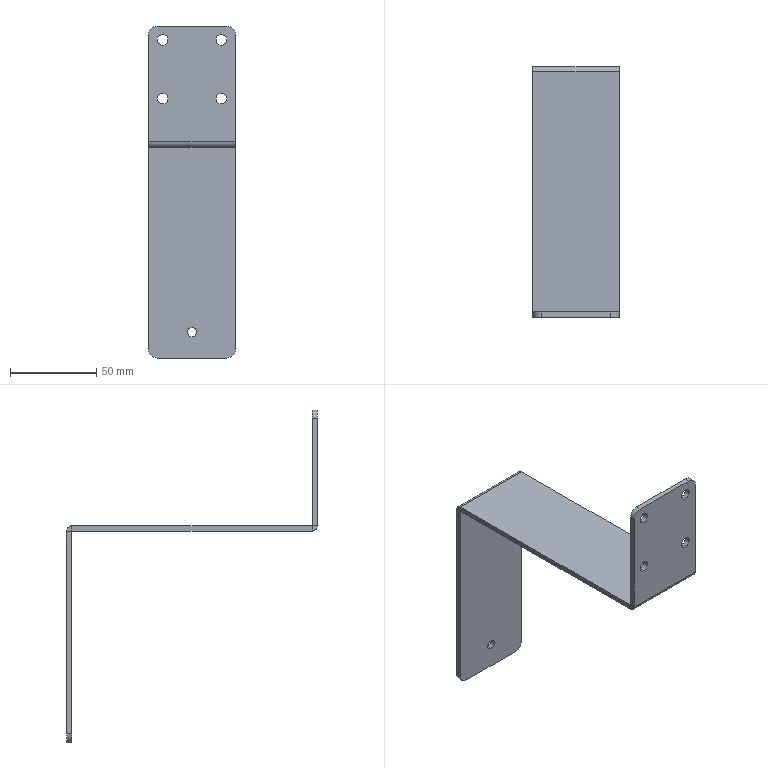Part | SolidWorks | features EdgeFlange 2, HoleWzd 2, Fillet 1, FlatPattern 1, SMBaseFlange 1, SheetMetal 1 | 1 solid | 36 faces | box 50 x 145 x 192 mm | volume 49401 mm3 | cylinder 18 | plane 18 | commonest cylinder face diameters 6.2 x10 10 x4 0.2 x2 5.3 x2
STEP:
#1=CARTESIAN_POINT('',(0.,139.,-139.35));
#2=VERTEX_POINT('',#1);
#3=CARTESIAN_POINT('',(0.,139.,-144.65));
#4=VERTEX_POINT('',#3);
#5=CARTESIAN_POINT('',(0.,139.,-142.));
#6=DIRECTION('',(0.,-1.,0.));
#7=DIRECTION('',(0.,0.,-1.));
#8=AXIS2_PLACEMENT_3D('',#5,#6,#7);
#9=CIRCLE('',#8,2.65);
#10=EDGE_CURVE('',#2,#4,#9,.T.);
#11=ORIENTED_EDGE('',*,*,#10,.T.);
#12=CARTESIAN_POINT('',(0.,142.,-144.65));
#13=VERTEX_POINT('',#12);
#14=CARTESIAN_POINT('',(0.,142.,-144.65));
#15=DIRECTION('',(0.,1.,0.));
#16=VECTOR('',#15,1000.);
#17=LINE('',#14,#16);
#18=EDGE_CURVE('',#4,#13,#17,.T.);
#19=ORIENTED_EDGE('',*,*,#18,.T.);
#20=CARTESIAN_POINT('',(0.,142.,-139.35));
#21=VERTEX_POINT('',#20);
#22=CARTESIAN_POINT('',(0.,142.,-142.));
#23=DIRECTION('',(0.,1.,0.));
#24=DIRECTION('',(0.,0.,1.));
#25=AXIS2_PLACEMENT_3D('',#22,#23,#24);
#26=CIRCLE('',#25,2.65);
#27=EDGE_CURVE('',#13,#21,#26,.T.);
#28=ORIENTED_EDGE('',*,*,#27,.T.);
#29=CARTESIAN_POINT('',(0.,142.,-139.35));
#30=DIRECTION('',(0.,1.,0.));
#31=VECTOR('',#30,1000.);
#32=LINE('',#29,#31);
#33=EDGE_CURVE('',#2,#21,#32,.T.);
#34=ORIENTED_EDGE('',*,*,#33,.F.);
#35=EDGE_LOOP('',(#11,#19,#28,#34));
#36=FACE_OUTER_BOUND('',#35,.T.);
#37=CARTESIAN_POINT('',(0.,142.,-142.));
#38=DIRECTION('',(0.,1.,0.));
#39=DIRECTION('',(0.,0.,1.));
#40=AXIS2_PLACEMENT_3D('',#37,#38,#39);
#41=CYLINDRICAL_SURFACE('',#40,2.65);
#42=ADVANCED_FACE('',(#36),#41,.F.);
#43=CARTESIAN_POINT('',(-17.,-3.,-3.9));
#44=VERTEX_POINT('',#43);
#45=CARTESIAN_POINT('',(-17.,-3.,-10.1));
#46=VERTEX_POINT('',#45);
#47=CARTESIAN_POINT('',(-17.,-3.,-7.));
#48=DIRECTION('',(0.,-1.,0.));
#49=DIRECTION('',(0.,0.,-1.));
#50=AXIS2_PLACEMENT_3D('',#47,#48,#49);
#51=CIRCLE('',#50,3.1);
#52=EDGE_CURVE('',#44,#46,#51,.T.);
#53=ORIENTED_EDGE('',*,*,#52,.T.);
#54=CARTESIAN_POINT('',(-17.,0.,-10.1));
#55=VERTEX_POINT('',#54);
#56=CARTESIAN_POINT('',(-17.,0.,-10.1));
#57=DIRECTION('',(0.,1.,0.));
#58=VECTOR('',#57,1000.);
#59=LINE('',#56,#58);
#60=EDGE_CURVE('',#46,#55,#59,.T.);
#61=ORIENTED_EDGE('',*,*,#60,.T.);
#62=CARTESIAN_POINT('',(-17.,0.,-3.9));
#63=VERTEX_POINT('',#62);
#64=CARTESIAN_POINT('',(-17.,0.,-7.));
#65=DIRECTION('',(0.,1.,0.));
#66=DIRECTION('',(0.,0.,1.));
#67=AXIS2_PLACEMENT_3D('',#64,#65,#66);
#68=CIRCLE('',#67,3.1);
#69=EDGE_CURVE('',#55,#63,#68,.T.);
#70=ORIENTED_EDGE('',*,*,#69,.T.);
#71=CARTESIAN_POINT('',(-17.,0.,-3.9));
#72=DIRECTION('',(0.,1.,0.));
#73=VECTOR('',#72,1000.);
#74=LINE('',#71,#73);
#75=EDGE_CURVE('',#44,#63,#74,.T.);
#76=ORIENTED_EDGE('',*,*,#75,.F.);
#77=EDGE_LOOP('',(#53,#61,#70,#76));
#78=FACE_OUTER_BOUND('',#77,.T.);
#79=CARTESIAN_POINT('',(-17.,0.,-7.));
#80=DIRECTION('',(0.,1.,0.));
#81=DIRECTION('',(0.,0.,1.));
#82=AXIS2_PLACEMENT_3D('',#79,#80,#81);
#83=CYLINDRICAL_SURFACE('',#82,3.1);
#84=ADVANCED_FACE('',(#78),#83,.F.);
#85=CARTESIAN_POINT('',(-17.,-3.,30.1));
#86=VERTEX_POINT('',#85);
#87=CARTESIAN_POINT('',(-17.,-3.,23.9));
#88=VERTEX_POINT('',#87);
#89=CARTESIAN_POINT('',(-17.,-3.,27.));
#90=DIRECTION('',(0.,-1.,0.));
#91=DIRECTION('',(0.,0.,-1.));
#92=AXIS2_PLACEMENT_3D('',#89,#90,#91);
#93=CIRCLE('',#92,3.1);
#94=EDGE_CURVE('',#86,#88,#93,.T.);
#95=ORIENTED_EDGE('',*,*,#94,.T.);
#96=CARTESIAN_POINT('',(-17.,0.,23.9));
#97=VERTEX_POINT('',#96);
#98=CARTESIAN_POINT('',(-17.,0.,23.9));
#99=DIRECTION('',(0.,1.,0.));
#100=VECTOR('',#99,1000.);
#101=LINE('',#98,#100);
#102=EDGE_CURVE('',#88,#97,#101,.T.);
#103=ORIENTED_EDGE('',*,*,#102,.T.);
#104=CARTESIAN_POINT('',(-17.,0.,30.1));
#105=VERTEX_POINT('',#104);
#106=CARTESIAN_POINT('',(-17.,0.,27.));
#107=DIRECTION('',(0.,1.,0.));
#108=DIRECTION('',(0.,0.,1.));
#109=AXIS2_PLACEMENT_3D('',#106,#107,#108);
#110=CIRCLE('',#109,3.1);
#111=EDGE_CURVE('',#97,#105,#110,.T.);
#112=ORIENTED_EDGE('',*,*,#111,.T.);
#113=CARTESIAN_POINT('',(-17.,0.,30.1));
#114=DIRECTION('',(0.,1.,0.));
#115=VECTOR('',#114,1000.);
#116=LINE('',#113,#115);
#117=EDGE_CURVE('',#86,#105,#116,.T.);
#118=ORIENTED_EDGE('',*,*,#117,.F.);
#119=EDGE_LOOP('',(#95,#103,#112,#118));
#120=FACE_OUTER_BOUND('',#119,.T.);
#121=CARTESIAN_POINT('',(-17.,0.,27.));
#122=DIRECTION('',(0.,1.,0.));
#123=DIRECTION('',(0.,0.,1.));
#124=AXIS2_PLACEMENT_3D('',#121,#122,#123);
#125=CYLINDRICAL_SURFACE('',#124,3.1);
#126=ADVANCED_FACE('',(#120),#125,.F.);
#127=CARTESIAN_POINT('',(17.,-3.,30.1));
#128=VERTEX_POINT('',#127);
#129=CARTESIAN_POINT('',(17.,-3.,23.9));
#130=VERTEX_POINT('',#129);
#131=CARTESIAN_POINT('',(17.,-3.,27.));
#132=DIRECTION('',(0.,-1.,0.));
#133=DIRECTION('',(0.,0.,-1.));
#134=AXIS2_PLACEMENT_3D('',#131,#132,#133);
#135=CIRCLE('',#134,3.1);
#136=EDGE_CURVE('',#128,#130,#135,.T.);
#137=ORIENTED_EDGE('',*,*,#136,.T.);
#138=CARTESIAN_POINT('',(17.,0.,23.9));
#139=VERTEX_POINT('',#138);
#140=CARTESIAN_POINT('',(17.,0.,23.9));
#141=DIRECTION('',(0.,1.,0.));
#142=VECTOR('',#141,1000.);
#143=LINE('',#140,#142);
#144=EDGE_CURVE('',#130,#139,#143,.T.);
#145=ORIENTED_EDGE('',*,*,#144,.T.);
#146=CARTESIAN_POINT('',(17.,0.,30.1));
#147=VERTEX_POINT('',#146);
#148=CARTESIAN_POINT('',(17.,0.,27.));
#149=DIRECTION('',(0.,1.,0.));
#150=DIRECTION('',(0.,0.,1.));
#151=AXIS2_PLACEMENT_3D('',#148,#149,#150);
#152=CIRCLE('',#151,3.1);
#153=EDGE_CURVE('',#139,#147,#152,.T.);
#154=ORIENTED_EDGE('',*,*,#153,.T.);
#155=CARTESIAN_POINT('',(17.,0.,30.1));
#156=DIRECTION('',(0.,1.,0.));
#157=VECTOR('',#156,1000.);
#158=LINE('',#155,#157);
#159=EDGE_CURVE('',#128,#147,#158,.T.);
#160=ORIENTED_EDGE('',*,*,#159,.F.);
#161=EDGE_LOOP('',(#137,#145,#154,#160));
#162=FACE_OUTER_BOUND('',#161,.T.);
#163=CARTESIAN_POINT('',(17.,0.,27.));
#164=DIRECTION('',(0.,1.,0.));
#165=DIRECTION('',(0.,0.,1.));
#166=AXIS2_PLACEMENT_3D('',#163,#164,#165);
#167=CYLINDRICAL_SURFACE('',#166,3.1);
#168=ADVANCED_FACE('',(#162),#167,.F.);
#169=CARTESIAN_POINT('',(17.,-3.,-3.9));
#170=VERTEX_POINT('',#169);
#171=CARTESIAN_POINT('',(17.,-3.,-10.1));
#172=VERTEX_POINT('',#171);
#173=CARTESIAN_POINT('',(17.,-3.,-7.));
#174=DIRECTION('',(0.,-1.,0.));
#175=DIRECTION('',(0.,0.,-1.));
#176=AXIS2_PLACEMENT_3D('',#173,#174,#175);
#177=CIRCLE('',#176,3.1);
#178=EDGE_CURVE('',#170,#172,#177,.T.);
#179=ORIENTED_EDGE('',*,*,#178,.T.);
#180=CARTESIAN_POINT('',(17.,0.,-10.1));
#181=VERTEX_POINT('',#180);
#182=CARTESIAN_POINT('',(17.,0.,-10.1));
#183=DIRECTION('',(0.,1.,0.));
#184=VECTOR('',#183,1000.);
#185=LINE('',#182,#184);
#186=EDGE_CURVE('',#172,#181,#185,.T.);
#187=ORIENTED_EDGE('',*,*,#186,.T.);
#188=CARTESIAN_POINT('',(17.,0.,-3.9));
#189=VERTEX_POINT('',#188);
#190=CARTESIAN_POINT('',(17.,0.,-7.));
#191=DIRECTION('',(0.,1.,0.));
#192=DIRECTION('',(0.,0.,1.));
#193=AXIS2_PLACEMENT_3D('',#190,#191,#192);
#194=CIRCLE('',#193,3.1);
#195=EDGE_CURVE('',#181,#189,#194,.T.);
#196=ORIENTED_EDGE('',*,*,#195,.T.);
#197=CARTESIAN_POINT('',(17.,0.,-3.9));
#198=DIRECTION('',(0.,1.,0.));
#199=VECTOR('',#198,1000.);
#200=LINE('',#197,#199);
#201=EDGE_CURVE('',#170,#189,#200,.T.);
#202=ORIENTED_EDGE('',*,*,#201,.F.);
#203=EDGE_LOOP('',(#179,#187,#196,#202));
#204=FACE_OUTER_BOUND('',#203,.T.);
#205=CARTESIAN_POINT('',(17.,0.,-7.));
#206=DIRECTION('',(0.,1.,0.));
#207=DIRECTION('',(0.,0.,1.));
#208=AXIS2_PLACEMENT_3D('',#205,#206,#207);
#209=CYLINDRICAL_SURFACE('',#208,3.1);
#210=ADVANCED_FACE('',(#204),#209,.F.);
#211=CARTESIAN_POINT('',(25.,138.9,-35.));
#212=VERTEX_POINT('',#211);
#213=CARTESIAN_POINT('',(25.,138.9,-32.));
#214=VERTEX_POINT('',#213);
#215=CARTESIAN_POINT('',(25.,138.9,-35.));
#216=DIRECTION('',(0.,0.,1.));
#217=VECTOR('',#216,1000.);
#218=LINE('',#215,#217);
#219=EDGE_CURVE('',#212,#214,#218,.T.);
#220=ORIENTED_EDGE('',*,*,#219,.T.);
#221=CARTESIAN_POINT('',(25.,0.1,-32.));
#222=VERTEX_POINT('',#221);
#223=CARTESIAN_POINT('',(25.,0.,-32.));
#224=DIRECTION('',(0.,-1.,0.));
#225=VECTOR('',#224,1000.);
#226=LINE('',#223,#225);
#227=EDGE_CURVE('',#214,#222,#226,.T.);
#228=ORIENTED_EDGE('',*,*,#227,.T.);
#229=CARTESIAN_POINT('',(25.,0.1,-35.));
#230=VERTEX_POINT('',#229);
#231=CARTESIAN_POINT('',(25.,0.1,-35.));
#232=DIRECTION('',(0.,0.,-1.));
#233=VECTOR('',#232,1000.);
#234=LINE('',#231,#233);
#235=EDGE_CURVE('',#222,#230,#234,.T.);
#236=ORIENTED_EDGE('',*,*,#235,.T.);
#237=CARTESIAN_POINT('',(25.,0.,-35.));
#238=DIRECTION('',(0.,-1.,0.));
#239=VECTOR('',#238,1000.);
#240=LINE('',#237,#239);
#241=EDGE_CURVE('',#212,#230,#240,.T.);
#242=ORIENTED_EDGE('',*,*,#241,.F.);
#243=EDGE_LOOP('',(#220,#228,#236,#242));
#244=FACE_OUTER_BOUND('',#243,.T.);
#245=CARTESIAN_POINT('',(25.,0.,-35.));
#246=DIRECTION('',(-1.,0.,0.));
#247=DIRECTION('',(0.,-1.,0.));
#248=AXIS2_PLACEMENT_3D('',#245,#246,#247);
#249=PLANE('',#248);
#250=ADVANCED_FACE('',(#244),#249,.F.);
#251=CARTESIAN_POINT('',(-25.,138.9,-35.));
#252=VERTEX_POINT('',#251);
#253=CARTESIAN_POINT('',(-25.,138.9,-32.));
#254=VERTEX_POINT('',#253);
#255=CARTESIAN_POINT('',(-25.,138.9,-35.));
#256=DIRECTION('',(0.,0.,1.));
#257=VECTOR('',#256,1000.);
#258=LINE('',#255,#257);
#259=EDGE_CURVE('',#252,#254,#258,.T.);
#260=ORIENTED_EDGE('',*,*,#259,.F.);
#261=CARTESIAN_POINT('',(-25.,0.1,-35.));
#262=VERTEX_POINT('',#261);
#263=CARTESIAN_POINT('',(-25.,0.,-35.));
#264=DIRECTION('',(0.,1.,0.));
#265=VECTOR('',#264,1000.);
#266=LINE('',#263,#265);
#267=EDGE_CURVE('',#262,#252,#266,.T.);
#268=ORIENTED_EDGE('',*,*,#267,.F.);
#269=CARTESIAN_POINT('',(-25.,0.1,-32.));
#270=VERTEX_POINT('',#269);
#271=CARTESIAN_POINT('',(-25.,0.1,-32.));
#272=DIRECTION('',(0.,0.,-1.));
#273=VECTOR('',#272,1000.);
#274=LINE('',#271,#273);
#275=EDGE_CURVE('',#270,#262,#274,.T.);
#276=ORIENTED_EDGE('',*,*,#275,.F.);
#277=CARTESIAN_POINT('',(-25.,142.,-32.));
#278=DIRECTION('',(0.,1.,0.));
#279=VECTOR('',#278,1000.);
#280=LINE('',#277,#279);
#281=EDGE_CURVE('',#270,#254,#280,.T.);
#282=ORIENTED_EDGE('',*,*,#281,.T.);
#283=EDGE_LOOP('',(#260,#268,#276,#282));
#284=FACE_OUTER_BOUND('',#283,.T.);
#285=CARTESIAN_POINT('',(-25.,142.,-35.));
#286=DIRECTION('',(1.,0.,0.));
#287=DIRECTION('',(0.,1.,0.));
#288=AXIS2_PLACEMENT_3D('',#285,#286,#287);
#289=PLANE('',#288);
#290=ADVANCED_FACE('',(#284),#289,.F.);
#291=CARTESIAN_POINT('',(25.,138.9,-35.));
#292=DIRECTION('',(-1.,0.,0.));
#293=VECTOR('',#292,1000.);
#294=LINE('',#291,#293);
#295=EDGE_CURVE('',#212,#252,#294,.T.);
#296=ORIENTED_EDGE('',*,*,#295,.F.);
#297=ORIENTED_EDGE('',*,*,#241,.T.);
#298=CARTESIAN_POINT('',(25.,0.1,-35.));
#299=DIRECTION('',(1.,0.,0.));
#300=VECTOR('',#299,1000.);
#301=LINE('',#298,#300);
#302=EDGE_CURVE('',#262,#230,#301,.T.);
#303=ORIENTED_EDGE('',*,*,#302,.F.);
#304=ORIENTED_EDGE('',*,*,#267,.T.);
#305=EDGE_LOOP('',(#296,#297,#303,#304));
#306=FACE_OUTER_BOUND('',#305,.T.);
#307=CARTESIAN_POINT('',(0.,0.,-35.));
#308=DIRECTION('',(0.,0.,1.));
#309=DIRECTION('',(0.,-1.,0.));
#310=AXIS2_PLACEMENT_3D('',#307,#308,#309);
#311=PLANE('',#310);
#312=ADVANCED_FACE('',(#306),#311,.F.);
#313=ORIENTED_EDGE('',*,*,#227,.F.);
#314=CARTESIAN_POINT('',(25.,138.9,-32.));
#315=DIRECTION('',(-1.,0.,0.));
#316=VECTOR('',#315,1000.);
#317=LINE('',#314,#316);
#318=EDGE_CURVE('',#214,#254,#317,.T.);
#319=ORIENTED_EDGE('',*,*,#318,.T.);
#320=ORIENTED_EDGE('',*,*,#281,.F.);
#321=CARTESIAN_POINT('',(25.,0.1,-32.));
#322=DIRECTION('',(-1.,0.,0.));
#323=VECTOR('',#322,1000.);
#324=LINE('',#321,#323);
#325=EDGE_CURVE('',#222,#270,#324,.T.);
#326=ORIENTED_EDGE('',*,*,#325,.F.);
#327=EDGE_LOOP('',(#313,#319,#320,#326));
#328=FACE_OUTER_BOUND('',#327,.T.);
#329=CARTESIAN_POINT('',(0.,0.,-32.));
#330=DIRECTION('',(0.,0.,1.));
#331=DIRECTION('',(0.,-1.,0.));
#332=AXIS2_PLACEMENT_3D('',#329,#330,#331);
#333=PLANE('',#332);
#334=ADVANCED_FACE('',(#328),#333,.T.);
#335=CARTESIAN_POINT('',(-17.,0.,27.));
#336=DIRECTION('',(0.,1.,0.));
#337=DIRECTION('',(0.,0.,1.));
#338=AXIS2_PLACEMENT_3D('',#335,#336,#337);
#339=CIRCLE('',#338,3.1);
#340=EDGE_CURVE('',#105,#97,#339,.T.);
#341=ORIENTED_EDGE('',*,*,#340,.F.);
#342=ORIENTED_EDGE('',*,*,#111,.F.);
#343=EDGE_LOOP('',(#341,#342));
#344=FACE_BOUND('',#343,.T.);
#345=CARTESIAN_POINT('',(17.,0.,-7.));
#346=DIRECTION('',(0.,1.,0.));
#347=DIRECTION('',(0.,0.,1.));
#348=AXIS2_PLACEMENT_3D('',#345,#346,#347);
#349=CIRCLE('',#348,3.1);
#350=EDGE_CURVE('',#189,#181,#349,.T.);
#351=ORIENTED_EDGE('',*,*,#350,.F.);
#352=ORIENTED_EDGE('',*,*,#195,.F.);
#353=EDGE_LOOP('',(#351,#352));
#354=FACE_BOUND('',#353,.T.);
#355=CARTESIAN_POINT('',(17.,0.,27.));
#356=DIRECTION('',(0.,1.,0.));
#357=DIRECTION('',(0.,0.,1.));
#358=AXIS2_PLACEMENT_3D('',#355,#356,#357);
#359=CIRCLE('',#358,3.1);
#360=EDGE_CURVE('',#147,#139,#359,.T.);
#361=ORIENTED_EDGE('',*,*,#360,.F.);
#362=ORIENTED_EDGE('',*,*,#153,.F.);
#363=EDGE_LOOP('',(#361,#362));
#364=FACE_BOUND('',#363,.T.);
#365=CARTESIAN_POINT('',(-17.,0.,-7.));
#366=DIRECTION('',(0.,1.,0.));
#367=DIRECTION('',(0.,0.,1.));
#368=AXIS2_PLACEMENT_3D('',#365,#366,#367);
#369=CIRCLE('',#368,3.1);
#370=EDGE_CURVE('',#63,#55,#369,.T.);
#371=ORIENTED_EDGE('',*,*,#370,.F.);
#372=ORIENTED_EDGE('',*,*,#69,.F.);
#373=EDGE_LOOP('',(#371,#372));
#374=FACE_BOUND('',#373,.T.);
#375=CARTESIAN_POINT('',(-20.,0.,35.));
#376=VERTEX_POINT('',#375);
#377=CARTESIAN_POINT('',(20.,0.,35.));
#378=VERTEX_POINT('',#377);
#379=CARTESIAN_POINT('',(-25.,0.,35.));
#380=DIRECTION('',(1.,0.,0.));
#381=VECTOR('',#380,1000.);
#382=LINE('',#379,#381);
#383=EDGE_CURVE('',#376,#378,#382,.T.);
#384=ORIENTED_EDGE('',*,*,#383,.T.);
#385=CARTESIAN_POINT('',(25.,0.,30.));
#386=VERTEX_POINT('',#385);
#387=CARTESIAN_POINT('',(20.,0.,30.));
#388=DIRECTION('',(0.,1.,0.));
#389=DIRECTION('',(0.,0.,-1.));
#390=AXIS2_PLACEMENT_3D('',#387,#388,#389);
#391=CIRCLE('',#390,5.);
#392=EDGE_CURVE('',#378,#386,#391,.T.);
#393=ORIENTED_EDGE('',*,*,#392,.T.);
#394=CARTESIAN_POINT('',(25.,0.,-31.9));
#395=VERTEX_POINT('',#394);
#396=CARTESIAN_POINT('',(25.,0.,35.));
#397=DIRECTION('',(0.,0.,-1.));
#398=VECTOR('',#397,1000.);
#399=LINE('',#396,#398);
#400=EDGE_CURVE('',#386,#395,#399,.T.);
#401=ORIENTED_EDGE('',*,*,#400,.T.);
#402=CARTESIAN_POINT('',(-25.,0.,-31.9));
#403=VERTEX_POINT('',#402);
#404=CARTESIAN_POINT('',(-25.,0.,-31.9));
#405=DIRECTION('',(1.,0.,0.));
#406=VECTOR('',#405,1000.);
#407=LINE('',#404,#406);
#408=EDGE_CURVE('',#403,#395,#407,.T.);
#409=ORIENTED_EDGE('',*,*,#408,.F.);
#410=CARTESIAN_POINT('',(-25.,0.,30.));
#411=VERTEX_POINT('',#410);
#412=CARTESIAN_POINT('',(-25.,0.,35.));
#413=DIRECTION('',(0.,0.,1.));
#414=VECTOR('',#413,1000.);
#415=LINE('',#412,#414);
#416=EDGE_CURVE('',#403,#411,#415,.T.);
#417=ORIENTED_EDGE('',*,*,#416,.T.);
#418=CARTESIAN_POINT('',(-20.,0.,30.));
#419=DIRECTION('',(0.,1.,0.));
#420=DIRECTION('',(0.,0.,-1.));
#421=AXIS2_PLACEMENT_3D('',#418,#419,#420);
#422=CIRCLE('',#421,5.);
#423=EDGE_CURVE('',#411,#376,#422,.T.);
#424=ORIENTED_EDGE('',*,*,#423,.T.);
#425=EDGE_LOOP('',(#384,#393,#401,#409,#417,#424));
#426=FACE_OUTER_BOUND('',#425,.T.);
#427=CARTESIAN_POINT('',(0.,0.,0.));
#428=DIRECTION('',(0.,-1.,0.));
#429=DIRECTION('',(0.,0.,-1.));
#430=AXIS2_PLACEMENT_3D('',#427,#428,#429);
#431=PLANE('',#430);
#432=ADVANCED_FACE('',(#344,#354,#364,#374,#426),#431,.F.);
#433=CARTESIAN_POINT('',(-25.,-3.,-31.9));
#434=VERTEX_POINT('',#433);
#435=CARTESIAN_POINT('',(-25.,-3.,30.));
#436=VERTEX_POINT('',#435);
#437=CARTESIAN_POINT('',(-25.,-3.,35.));
#438=DIRECTION('',(0.,0.,1.));
#439=VECTOR('',#438,1000.);
#440=LINE('',#437,#439);
#441=EDGE_CURVE('',#434,#436,#440,.T.);
#442=ORIENTED_EDGE('',*,*,#441,.T.);
#443=CARTESIAN_POINT('',(-25.,-3.,30.));
#444=DIRECTION('',(0.,1.,0.));
#445=VECTOR('',#444,1000.);
#446=LINE('',#443,#445);
#447=EDGE_CURVE('',#436,#411,#446,.T.);
#448=ORIENTED_EDGE('',*,*,#447,.T.);
#449=ORIENTED_EDGE('',*,*,#416,.F.);
#450=CARTESIAN_POINT('',(-25.,0.,-31.9));
#451=DIRECTION('',(0.,-1.,0.));
#452=VECTOR('',#451,1000.);
#453=LINE('',#450,#452);
#454=EDGE_CURVE('',#403,#434,#453,.T.);
#455=ORIENTED_EDGE('',*,*,#454,.T.);
#456=EDGE_LOOP('',(#442,#448,#449,#455));
#457=FACE_OUTER_BOUND('',#456,.T.);
#458=CARTESIAN_POINT('',(-25.,-3.,35.));
#459=DIRECTION('',(-1.,0.,0.));
#460=DIRECTION('',(0.,0.,1.));
#461=AXIS2_PLACEMENT_3D('',#458,#459,#460);
#462=PLANE('',#461);
#463=ADVANCED_FACE('',(#457),#462,.T.);
#464=ORIENTED_EDGE('',*,*,#52,.F.);
#465=CARTESIAN_POINT('',(-17.,-3.,-7.));
#466=DIRECTION('',(0.,-1.,0.));
#467=DIRECTION('',(0.,0.,-1.));
#468=AXIS2_PLACEMENT_3D('',#465,#466,#467);
#469=CIRCLE('',#468,3.1);
#470=EDGE_CURVE('',#46,#44,#469,.T.);
#471=ORIENTED_EDGE('',*,*,#470,.F.);
#472=EDGE_LOOP('',(#464,#471));
#473=FACE_BOUND('',#472,.T.);
#474=ORIENTED_EDGE('',*,*,#94,.F.);
#475=CARTESIAN_POINT('',(-17.,-3.,27.));
#476=DIRECTION('',(0.,-1.,0.));
#477=DIRECTION('',(0.,0.,-1.));
#478=AXIS2_PLACEMENT_3D('',#475,#476,#477);
#479=CIRCLE('',#478,3.1);
#480=EDGE_CURVE('',#88,#86,#479,.T.);
#481=ORIENTED_EDGE('',*,*,#480,.F.);
#482=EDGE_LOOP('',(#474,#481));
#483=FACE_BOUND('',#482,.T.);
#484=ORIENTED_EDGE('',*,*,#136,.F.);
#485=CARTESIAN_POINT('',(17.,-3.,27.));
#486=DIRECTION('',(0.,-1.,0.));
#487=DIRECTION('',(0.,0.,-1.));
#488=AXIS2_PLACEMENT_3D('',#485,#486,#487);
#489=CIRCLE('',#488,3.1);
#490=EDGE_CURVE('',#130,#128,#489,.T.);
#491=ORIENTED_EDGE('',*,*,#490,.F.);
#492=EDGE_LOOP('',(#484,#491));
#493=FACE_BOUND('',#492,.T.);
#494=ORIENTED_EDGE('',*,*,#178,.F.);
#495=CARTESIAN_POINT('',(17.,-3.,-7.));
#496=DIRECTION('',(0.,-1.,0.));
#497=DIRECTION('',(0.,0.,-1.));
#498=AXIS2_PLACEMENT_3D('',#495,#496,#497);
#499=CIRCLE('',#498,3.1);
#500=EDGE_CURVE('',#172,#170,#499,.T.);
#501=ORIENTED_EDGE('',*,*,#500,.F.);
#502=EDGE_LOOP('',(#494,#501));
#503=FACE_BOUND('',#502,.T.);
#504=CARTESIAN_POINT('',(25.,-3.,30.));
#505=VERTEX_POINT('',#504);
#506=CARTESIAN_POINT('',(25.,-3.,-31.9));
#507=VERTEX_POINT('',#506);
#508=CARTESIAN_POINT('',(25.,-3.,35.));
#509=DIRECTION('',(0.,0.,-1.));
#510=VECTOR('',#509,1000.);
#511=LINE('',#508,#510);
#512=EDGE_CURVE('',#505,#507,#511,.T.);
#513=ORIENTED_EDGE('',*,*,#512,.F.);
#514=CARTESIAN_POINT('',(20.,-3.,35.));
#515=VERTEX_POINT('',#514);
#516=CARTESIAN_POINT('',(20.,-3.,30.));
#517=DIRECTION('',(0.,-1.,0.));
#518=DIRECTION('',(0.,0.,-1.));
#519=AXIS2_PLACEMENT_3D('',#516,#517,#518);
#520=CIRCLE('',#519,5.);
#521=EDGE_CURVE('',#505,#515,#520,.T.);
#522=ORIENTED_EDGE('',*,*,#521,.T.);
#523=CARTESIAN_POINT('',(-20.,-3.,35.));
#524=VERTEX_POINT('',#523);
#525=CARTESIAN_POINT('',(-25.,-3.,35.));
#526=DIRECTION('',(1.,0.,0.));
#527=VECTOR('',#526,1000.);
#528=LINE('',#525,#527);
#529=EDGE_CURVE('',#524,#515,#528,.T.);
#530=ORIENTED_EDGE('',*,*,#529,.F.);
#531=CARTESIAN_POINT('',(-20.,-3.,30.));
#532=DIRECTION('',(0.,-1.,0.));
#533=DIRECTION('',(0.,0.,-1.));
#534=AXIS2_PLACEMENT_3D('',#531,#532,#533);
#535=CIRCLE('',#534,5.);
#536=EDGE_CURVE('',#524,#436,#535,.T.);
#537=ORIENTED_EDGE('',*,*,#536,.T.);
#538=ORIENTED_EDGE('',*,*,#441,.F.);
#539=CARTESIAN_POINT('',(-25.,-3.,-31.9));
#540=DIRECTION('',(1.,0.,0.));
#541=VECTOR('',#540,1000.);
#542=LINE('',#539,#541);
#543=EDGE_CURVE('',#434,#507,#542,.T.);
#544=ORIENTED_EDGE('',*,*,#543,.T.);
#545=EDGE_LOOP('',(#513,#522,#530,#537,#538,#544));
#546=FACE_OUTER_BOUND('',#545,.T.);
#547=CARTESIAN_POINT('',(0.,-3.,0.));
#548=DIRECTION('',(0.,-1.,0.));
#549=DIRECTION('',(0.,0.,-1.));
#550=AXIS2_PLACEMENT_3D('',#547,#548,#549);
#551=PLANE('',#550);
#552=ADVANCED_FACE('',(#473,#483,#493,#503,#546),#551,.T.);
#553=ORIENTED_EDGE('',*,*,#400,.F.);
#554=CARTESIAN_POINT('',(25.,-3.,30.));
#555=DIRECTION('',(0.,-1.,0.));
#556=VECTOR('',#555,1000.);
#557=LINE('',#554,#556);
#558=EDGE_CURVE('',#386,#505,#557,.T.);
#559=ORIENTED_EDGE('',*,*,#558,.T.);
#560=ORIENTED_EDGE('',*,*,#512,.T.);
#561=CARTESIAN_POINT('',(25.,0.,-31.9));
#562=DIRECTION('',(0.,-1.,0.));
#563=VECTOR('',#562,1000.);
#564=LINE('',#561,#563);
#565=EDGE_CURVE('',#395,#507,#564,.T.);
#566=ORIENTED_EDGE('',*,*,#565,.F.);
#567=EDGE_LOOP('',(#553,#559,#560,#566));
#568=FACE_OUTER_BOUND('',#567,.T.);
#569=CARTESIAN_POINT('',(25.,-3.,35.));
#570=DIRECTION('',(1.,0.,0.));
#571=DIRECTION('',(0.,0.,-1.));
#572=AXIS2_PLACEMENT_3D('',#569,#570,#571);
#573=PLANE('',#572);
#574=ADVANCED_FACE('',(#568),#573,.T.);
#575=ORIENTED_EDGE('',*,*,#529,.T.);
#576=CARTESIAN_POINT('',(20.,-3.,35.));
#577=DIRECTION('',(0.,1.,0.));
#578=VECTOR('',#577,1000.);
#579=LINE('',#576,#578);
#580=EDGE_CURVE('',#515,#378,#579,.T.);
#581=ORIENTED_EDGE('',*,*,#580,.T.);
#582=ORIENTED_EDGE('',*,*,#383,.F.);
#583=CARTESIAN_POINT('',(-20.,-3.,35.));
#584=DIRECTION('',(0.,-1.,0.));
#585=VECTOR('',#584,1000.);
#586=LINE('',#583,#585);
#587=EDGE_CURVE('',#376,#524,#586,.T.);
#588=ORIENTED_EDGE('',*,*,#587,.T.);
#589=EDGE_LOOP('',(#575,#581,#582,#588));
#590=FACE_OUTER_BOUND('',#589,.T.);
#591=CARTESIAN_POINT('',(-25.,-3.,35.));
#592=DIRECTION('',(0.,0.,1.));
#593=DIRECTION('',(1.,0.,0.));
#594=AXIS2_PLACEMENT_3D('',#591,#592,#593);
#595=PLANE('',#594);
#596=ADVANCED_FACE('',(#590),#595,.T.);
#597=ORIENTED_EDGE('',*,*,#186,.F.);
#598=ORIENTED_EDGE('',*,*,#500,.T.);
#599=ORIENTED_EDGE('',*,*,#201,.T.);
#600=ORIENTED_EDGE('',*,*,#350,.T.);
#601=EDGE_LOOP('',(#597,#598,#599,#600));
#602=FACE_OUTER_BOUND('',#601,.T.);
#603=CARTESIAN_POINT('',(17.,0.,-7.));
#604=DIRECTION('',(0.,1.,0.));
#605=DIRECTION('',(0.,0.,1.));
#606=AXIS2_PLACEMENT_3D('',#603,#604,#605);
#607=CYLINDRICAL_SURFACE('',#606,3.1);
#608=ADVANCED_FACE('',(#602),#607,.F.);
#609=ORIENTED_EDGE('',*,*,#144,.F.);
#610=ORIENTED_EDGE('',*,*,#490,.T.);
#611=ORIENTED_EDGE('',*,*,#159,.T.);
#612=ORIENTED_EDGE('',*,*,#360,.T.);
#613=EDGE_LOOP('',(#609,#610,#611,#612));
#614=FACE_OUTER_BOUND('',#613,.T.);
#615=CARTESIAN_POINT('',(17.,0.,27.));
#616=DIRECTION('',(0.,1.,0.));
#617=DIRECTION('',(0.,0.,1.));
#618=AXIS2_PLACEMENT_3D('',#615,#616,#617);
#619=CYLINDRICAL_SURFACE('',#618,3.1);
#620=ADVANCED_FACE('',(#614),#619,.F.);
#621=ORIENTED_EDGE('',*,*,#102,.F.);
#622=ORIENTED_EDGE('',*,*,#480,.T.);
#623=ORIENTED_EDGE('',*,*,#117,.T.);
#624=ORIENTED_EDGE('',*,*,#340,.T.);
#625=EDGE_LOOP('',(#621,#622,#623,#624));
#626=FACE_OUTER_BOUND('',#625,.T.);
#627=CARTESIAN_POINT('',(-17.,0.,27.));
#628=DIRECTION('',(0.,1.,0.));
#629=DIRECTION('',(0.,0.,1.));
#630=AXIS2_PLACEMENT_3D('',#627,#628,#629);
#631=CYLINDRICAL_SURFACE('',#630,3.1);
#632=ADVANCED_FACE('',(#626),#631,.F.);
#633=ORIENTED_EDGE('',*,*,#60,.F.);
#634=ORIENTED_EDGE('',*,*,#470,.T.);
#635=ORIENTED_EDGE('',*,*,#75,.T.);
#636=ORIENTED_EDGE('',*,*,#370,.T.);
#637=EDGE_LOOP('',(#633,#634,#635,#636));
#638=FACE_OUTER_BOUND('',#637,.T.);
#639=CARTESIAN_POINT('',(-17.,0.,-7.));
#640=DIRECTION('',(0.,1.,0.));
#641=DIRECTION('',(0.,0.,1.));
#642=AXIS2_PLACEMENT_3D('',#639,#640,#641);
#643=CYLINDRICAL_SURFACE('',#642,3.1);
#644=ADVANCED_FACE('',(#638),#643,.F.);
#645=ORIENTED_EDGE('',*,*,#235,.F.);
#646=CARTESIAN_POINT('',(25.,0.1,-31.9));
#647=DIRECTION('',(1.,0.,0.));
#648=DIRECTION('',(0.,0.,1.));
#649=AXIS2_PLACEMENT_3D('',#646,#647,#648);
#650=CIRCLE('',#649,0.1);
#651=EDGE_CURVE('',#395,#222,#650,.T.);
#652=ORIENTED_EDGE('',*,*,#651,.F.);
#653=ORIENTED_EDGE('',*,*,#565,.T.);
#654=CARTESIAN_POINT('',(25.,0.1,-31.9));
#655=DIRECTION('',(1.,0.,0.));
#656=DIRECTION('',(0.,0.,1.));
#657=AXIS2_PLACEMENT_3D('',#654,#655,#656);
#658=CIRCLE('',#657,3.1);
#659=EDGE_CURVE('',#507,#230,#658,.T.);
#660=ORIENTED_EDGE('',*,*,#659,.T.);
#661=EDGE_LOOP('',(#645,#652,#653,#660));
#662=FACE_OUTER_BOUND('',#661,.T.);
#663=CARTESIAN_POINT('',(25.,0.1,-31.9));
#664=DIRECTION('',(1.,0.,0.));
#665=DIRECTION('',(0.,0.,-1.));
#666=AXIS2_PLACEMENT_3D('',#663,#664,#665);
#667=PLANE('',#666);
#668=ADVANCED_FACE('',(#662),#667,.T.);
#669=CARTESIAN_POINT('',(-25.,0.1,-31.9));
#670=DIRECTION('',(-1.,0.,0.));
#671=DIRECTION('',(0.,0.,1.));
#672=AXIS2_PLACEMENT_3D('',#669,#670,#671);
#673=CIRCLE('',#672,0.1);
#674=EDGE_CURVE('',#270,#403,#673,.T.);
#675=ORIENTED_EDGE('',*,*,#674,.F.);
#676=ORIENTED_EDGE('',*,*,#275,.T.);
#677=CARTESIAN_POINT('',(-25.,0.1,-31.9));
#678=DIRECTION('',(-1.,0.,0.));
#679=DIRECTION('',(0.,0.,1.));
#680=AXIS2_PLACEMENT_3D('',#677,#678,#679);
#681=CIRCLE('',#680,3.1);
#682=EDGE_CURVE('',#262,#434,#681,.T.);
#683=ORIENTED_EDGE('',*,*,#682,.T.);
#684=ORIENTED_EDGE('',*,*,#454,.F.);
#685=EDGE_LOOP('',(#675,#676,#683,#684));
#686=FACE_OUTER_BOUND('',#685,.T.);
#687=CARTESIAN_POINT('',(-25.,0.1,-31.9));
#688=DIRECTION('',(1.,0.,0.));
#689=DIRECTION('',(0.,0.,-1.));
#690=AXIS2_PLACEMENT_3D('',#687,#688,#689);
#691=PLANE('',#690);
#692=ADVANCED_FACE('',(#686),#691,.F.);
#693=ORIENTED_EDGE('',*,*,#543,.F.);
#694=ORIENTED_EDGE('',*,*,#682,.F.);
#695=ORIENTED_EDGE('',*,*,#302,.T.);
#696=ORIENTED_EDGE('',*,*,#659,.F.);
#697=EDGE_LOOP('',(#693,#694,#695,#696));
#698=FACE_OUTER_BOUND('',#697,.T.);
#699=CARTESIAN_POINT('',(-25.,0.1,-31.9));
#700=DIRECTION('',(-1.,0.,0.));
#701=DIRECTION('',(0.,0.,-1.));
#702=AXIS2_PLACEMENT_3D('',#699,#700,#701);
#703=CYLINDRICAL_SURFACE('',#702,3.1);
#704=ADVANCED_FACE('',(#698),#703,.T.);
#705=ORIENTED_EDGE('',*,*,#408,.T.);
#706=ORIENTED_EDGE('',*,*,#651,.T.);
#707=ORIENTED_EDGE('',*,*,#325,.T.);
#708=ORIENTED_EDGE('',*,*,#674,.T.);
#709=EDGE_LOOP('',(#705,#706,#707,#708));
#710=FACE_OUTER_BOUND('',#709,.T.);
#711=CARTESIAN_POINT('',(-25.,0.1,-31.9));
#712=DIRECTION('',(-1.,0.,0.));
#713=DIRECTION('',(0.,0.,-1.));
#714=AXIS2_PLACEMENT_3D('',#711,#712,#713);
#715=CYLINDRICAL_SURFACE('',#714,0.1);
#716=ADVANCED_FACE('',(#710),#715,.F.);
#717=CARTESIAN_POINT('',(-25.,139.,-35.1));
#718=VERTEX_POINT('',#717);
#719=CARTESIAN_POINT('',(-25.,142.,-35.1));
#720=VERTEX_POINT('',#719);
#721=CARTESIAN_POINT('',(-25.,142.,-35.1));
#722=DIRECTION('',(0.,1.,0.));
#723=VECTOR('',#722,1000.);
#724=LINE('',#721,#723);
#725=EDGE_CURVE('',#718,#720,#724,.T.);
#726=ORIENTED_EDGE('',*,*,#725,.F.);
#727=CARTESIAN_POINT('',(-25.,138.9,-35.1));
#728=DIRECTION('',(-1.,0.,0.));
#729=DIRECTION('',(0.,0.,-1.));
#730=AXIS2_PLACEMENT_3D('',#727,#728,#729);
#731=CIRCLE('',#730,0.1);
#732=EDGE_CURVE('',#252,#718,#731,.T.);
#733=ORIENTED_EDGE('',*,*,#732,.F.);
#734=ORIENTED_EDGE('',*,*,#259,.T.);
#735=CARTESIAN_POINT('',(-25.,138.9,-35.1));
#736=DIRECTION('',(-1.,0.,0.));
#737=DIRECTION('',(0.,0.,-1.));
#738=AXIS2_PLACEMENT_3D('',#735,#736,#737);
#739=CIRCLE('',#738,3.1);
#740=EDGE_CURVE('',#254,#720,#739,.T.);
#741=ORIENTED_EDGE('',*,*,#740,.T.);
#742=EDGE_LOOP('',(#726,#733,#734,#741));
#743=FACE_OUTER_BOUND('',#742,.T.);
#744=CARTESIAN_POINT('',(-25.,138.9,-35.1));
#745=DIRECTION('',(-1.,0.,0.));
#746=DIRECTION('',(0.,0.,1.));
#747=AXIS2_PLACEMENT_3D('',#744,#745,#746);
#748=PLANE('',#747);
#749=ADVANCED_FACE('',(#743),#748,.T.);
#750=CARTESIAN_POINT('',(25.,139.,-35.1));
#751=VERTEX_POINT('',#750);
#752=CARTESIAN_POINT('',(25.,138.9,-35.1));
#753=DIRECTION('',(1.,0.,0.));
#754=DIRECTION('',(0.,0.,-1.));
#755=AXIS2_PLACEMENT_3D('',#752,#753,#754);
#756=CIRCLE('',#755,0.1);
#757=EDGE_CURVE('',#751,#212,#756,.T.);
#758=ORIENTED_EDGE('',*,*,#757,.F.);
#759=CARTESIAN_POINT('',(25.,142.,-35.1));
#760=VERTEX_POINT('',#759);
#761=CARTESIAN_POINT('',(25.,139.,-35.1));
#762=DIRECTION('',(0.,1.,0.));
#763=VECTOR('',#762,1000.);
#764=LINE('',#761,#763);
#765=EDGE_CURVE('',#751,#760,#764,.T.);
#766=ORIENTED_EDGE('',*,*,#765,.T.);
#767=CARTESIAN_POINT('',(25.,138.9,-35.1));
#768=DIRECTION('',(1.,0.,0.));
#769=DIRECTION('',(0.,0.,-1.));
#770=AXIS2_PLACEMENT_3D('',#767,#768,#769);
#771=CIRCLE('',#770,3.1);
#772=EDGE_CURVE('',#760,#214,#771,.T.);
#773=ORIENTED_EDGE('',*,*,#772,.T.);
#774=ORIENTED_EDGE('',*,*,#219,.F.);
#775=EDGE_LOOP('',(#758,#766,#773,#774));
#776=FACE_OUTER_BOUND('',#775,.T.);
#777=CARTESIAN_POINT('',(25.,138.9,-35.1));
#778=DIRECTION('',(-1.,0.,0.));
#779=DIRECTION('',(0.,0.,1.));
#780=AXIS2_PLACEMENT_3D('',#777,#778,#779);
#781=PLANE('',#780);
#782=ADVANCED_FACE('',(#776),#781,.F.);
#783=ORIENTED_EDGE('',*,*,#318,.F.);
#784=ORIENTED_EDGE('',*,*,#772,.F.);
#785=CARTESIAN_POINT('',(-25.,142.,-35.1));
#786=DIRECTION('',(-1.,0.,0.));
#787=VECTOR('',#786,1000.);
#788=LINE('',#785,#787);
#789=EDGE_CURVE('',#760,#720,#788,.T.);
#790=ORIENTED_EDGE('',*,*,#789,.T.);
#791=ORIENTED_EDGE('',*,*,#740,.F.);
#792=EDGE_LOOP('',(#783,#784,#790,#791));
#793=FACE_OUTER_BOUND('',#792,.T.);
#794=CARTESIAN_POINT('',(25.,138.9,-35.1));
#795=DIRECTION('',(1.,0.,0.));
#796=DIRECTION('',(0.,1.,0.));
#797=AXIS2_PLACEMENT_3D('',#794,#795,#796);
#798=CYLINDRICAL_SURFACE('',#797,3.1);
#799=ADVANCED_FACE('',(#793),#798,.T.);
#800=ORIENTED_EDGE('',*,*,#295,.T.);
#801=ORIENTED_EDGE('',*,*,#732,.T.);
#802=CARTESIAN_POINT('',(-25.,139.,-35.1));
#803=DIRECTION('',(1.,0.,0.));
#804=VECTOR('',#803,1000.);
#805=LINE('',#802,#804);
#806=EDGE_CURVE('',#718,#751,#805,.T.);
#807=ORIENTED_EDGE('',*,*,#806,.T.);
#808=ORIENTED_EDGE('',*,*,#757,.T.);
#809=EDGE_LOOP('',(#800,#801,#807,#808));
#810=FACE_OUTER_BOUND('',#809,.T.);
#811=CARTESIAN_POINT('',(25.,138.9,-35.1));
#812=DIRECTION('',(1.,0.,0.));
#813=DIRECTION('',(0.,1.,0.));
#814=AXIS2_PLACEMENT_3D('',#811,#812,#813);
#815=CYLINDRICAL_SURFACE('',#814,0.1);
#816=ADVANCED_FACE('',(#810),#815,.F.);
#817=CARTESIAN_POINT('',(-25.,142.,-152.));
#818=VERTEX_POINT('',#817);
#819=CARTESIAN_POINT('',(-25.,142.,0.));
#820=DIRECTION('',(0.,0.,1.));
#821=VECTOR('',#820,1000.);
#822=LINE('',#819,#821);
#823=EDGE_CURVE('',#818,#720,#822,.T.);
#824=ORIENTED_EDGE('',*,*,#823,.F.);
#825=CARTESIAN_POINT('',(-25.,139.,-152.));
#826=VERTEX_POINT('',#825);
#827=CARTESIAN_POINT('',(-25.,142.,-152.));
#828=DIRECTION('',(0.,-1.,0.));
#829=VECTOR('',#828,1000.);
#830=LINE('',#827,#829);
#831=EDGE_CURVE('',#818,#826,#830,.T.);
#832=ORIENTED_EDGE('',*,*,#831,.T.);
#833=CARTESIAN_POINT('',(-25.,139.,-35.));
#834=DIRECTION('',(0.,0.,1.));
#835=VECTOR('',#834,1000.);
#836=LINE('',#833,#835);
#837=EDGE_CURVE('',#826,#718,#836,.T.);
#838=ORIENTED_EDGE('',*,*,#837,.T.);
#839=ORIENTED_EDGE('',*,*,#725,.T.);
#840=EDGE_LOOP('',(#824,#832,#838,#839));
#841=FACE_OUTER_BOUND('',#840,.T.);
#842=CARTESIAN_POINT('',(-25.,142.,-35.));
#843=DIRECTION('',(1.,0.,0.));
#844=DIRECTION('',(0.,0.,-1.));
#845=AXIS2_PLACEMENT_3D('',#842,#843,#844);
#846=PLANE('',#845);
#847=ADVANCED_FACE('',(#841),#846,.F.);
#848=CARTESIAN_POINT('',(25.,139.,-152.));
#849=VERTEX_POINT('',#848);
#850=CARTESIAN_POINT('',(25.,139.,-157.));
#851=DIRECTION('',(0.,0.,-1.));
#852=VECTOR('',#851,1000.);
#853=LINE('',#850,#852);
#854=EDGE_CURVE('',#751,#849,#853,.T.);
#855=ORIENTED_EDGE('',*,*,#854,.T.);
#856=CARTESIAN_POINT('',(25.,142.,-152.));
#857=VERTEX_POINT('',#856);
#858=CARTESIAN_POINT('',(25.,142.,-152.));
#859=DIRECTION('',(0.,1.,0.));
#860=VECTOR('',#859,1000.);
#861=LINE('',#858,#860);
#862=EDGE_CURVE('',#849,#857,#861,.T.);
#863=ORIENTED_EDGE('',*,*,#862,.T.);
#864=CARTESIAN_POINT('',(25.,142.,0.));
#865=DIRECTION('',(0.,0.,-1.));
#866=VECTOR('',#865,1000.);
#867=LINE('',#864,#866);
#868=EDGE_CURVE('',#760,#857,#867,.T.);
#869=ORIENTED_EDGE('',*,*,#868,.F.);
#870=ORIENTED_EDGE('',*,*,#765,.F.);
#871=EDGE_LOOP('',(#855,#863,#869,#870));
#872=FACE_OUTER_BOUND('',#871,.T.);
#873=CARTESIAN_POINT('',(25.,142.,-157.));
#874=DIRECTION('',(-1.,0.,0.));
#875=DIRECTION('',(0.,0.,1.));
#876=AXIS2_PLACEMENT_3D('',#873,#874,#875);
#877=PLANE('',#876);
#878=ADVANCED_FACE('',(#872),#877,.F.);
#879=CARTESIAN_POINT('',(0.,142.,-142.));
#880=DIRECTION('',(0.,1.,0.));
#881=DIRECTION('',(0.,0.,1.));
#882=AXIS2_PLACEMENT_3D('',#879,#880,#881);
#883=CIRCLE('',#882,2.65);
#884=EDGE_CURVE('',#21,#13,#883,.T.);
#885=ORIENTED_EDGE('',*,*,#884,.F.);
#886=ORIENTED_EDGE('',*,*,#27,.F.);
#887=EDGE_LOOP('',(#885,#886));
#888=FACE_BOUND('',#887,.T.);
#889=ORIENTED_EDGE('',*,*,#868,.T.);
#890=CARTESIAN_POINT('',(20.,142.,-157.));
#891=VERTEX_POINT('',#890);
#892=CARTESIAN_POINT('',(20.,142.,-152.));
#893=DIRECTION('',(0.,1.,0.));
#894=DIRECTION('',(0.,0.,-1.));
#895=AXIS2_PLACEMENT_3D('',#892,#893,#894);
#896=CIRCLE('',#895,5.);
#897=EDGE_CURVE('',#857,#891,#896,.T.);
#898=ORIENTED_EDGE('',*,*,#897,.T.);
#899=CARTESIAN_POINT('',(-20.,142.,-157.));
#900=VERTEX_POINT('',#899);
#901=CARTESIAN_POINT('',(0.,142.,-157.));
#902=DIRECTION('',(-1.,0.,0.));
#903=VECTOR('',#902,1000.);
#904=LINE('',#901,#903);
#905=EDGE_CURVE('',#891,#900,#904,.T.);
#906=ORIENTED_EDGE('',*,*,#905,.T.);
#907=CARTESIAN_POINT('',(-20.,142.,-152.));
#908=DIRECTION('',(0.,1.,0.));
#909=DIRECTION('',(0.,0.,-1.));
#910=AXIS2_PLACEMENT_3D('',#907,#908,#909);
#911=CIRCLE('',#910,5.);
#912=EDGE_CURVE('',#900,#818,#911,.T.);
#913=ORIENTED_EDGE('',*,*,#912,.T.);
#914=ORIENTED_EDGE('',*,*,#823,.T.);
#915=ORIENTED_EDGE('',*,*,#789,.F.);
#916=EDGE_LOOP('',(#889,#898,#906,#913,#914,#915));
#917=FACE_OUTER_BOUND('',#916,.T.);
#918=CARTESIAN_POINT('',(0.,142.,0.));
#919=DIRECTION('',(0.,-1.,0.));
#920=DIRECTION('',(0.,0.,-1.));
#921=AXIS2_PLACEMENT_3D('',#918,#919,#920);
#922=PLANE('',#921);
#923=ADVANCED_FACE('',(#888,#917),#922,.F.);
#924=ORIENTED_EDGE('',*,*,#10,.F.);
#925=CARTESIAN_POINT('',(0.,139.,-142.));
#926=DIRECTION('',(0.,-1.,0.));
#927=DIRECTION('',(0.,0.,-1.));
#928=AXIS2_PLACEMENT_3D('',#925,#926,#927);
#929=CIRCLE('',#928,2.65);
#930=EDGE_CURVE('',#4,#2,#929,.T.);
#931=ORIENTED_EDGE('',*,*,#930,.F.);
#932=EDGE_LOOP('',(#924,#931));
#933=FACE_BOUND('',#932,.T.);
#934=CARTESIAN_POINT('',(20.,139.,-157.));
#935=VERTEX_POINT('',#934);
#936=CARTESIAN_POINT('',(-20.,139.,-157.));
#937=VERTEX_POINT('',#936);
#938=CARTESIAN_POINT('',(-25.,139.,-157.));
#939=DIRECTION('',(-1.,0.,0.));
#940=VECTOR('',#939,1000.);
#941=LINE('',#938,#940);
#942=EDGE_CURVE('',#935,#937,#941,.T.);
#943=ORIENTED_EDGE('',*,*,#942,.F.);
#944=CARTESIAN_POINT('',(20.,139.,-152.));
#945=DIRECTION('',(0.,-1.,0.));
#946=DIRECTION('',(0.,0.,-1.));
#947=AXIS2_PLACEMENT_3D('',#944,#945,#946);
#948=CIRCLE('',#947,5.);
#949=EDGE_CURVE('',#935,#849,#948,.T.);
#950=ORIENTED_EDGE('',*,*,#949,.T.);
#951=ORIENTED_EDGE('',*,*,#854,.F.);
#952=ORIENTED_EDGE('',*,*,#806,.F.);
#953=ORIENTED_EDGE('',*,*,#837,.F.);
#954=CARTESIAN_POINT('',(-20.,139.,-152.));
#955=DIRECTION('',(0.,-1.,0.));
#956=DIRECTION('',(0.,0.,-1.));
#957=AXIS2_PLACEMENT_3D('',#954,#955,#956);
#958=CIRCLE('',#957,5.);
#959=EDGE_CURVE('',#826,#937,#958,.T.);
#960=ORIENTED_EDGE('',*,*,#959,.T.);
#961=EDGE_LOOP('',(#943,#950,#951,#952,#953,#960));
#962=FACE_OUTER_BOUND('',#961,.T.);
#963=CARTESIAN_POINT('',(0.,139.,0.));
#964=DIRECTION('',(0.,-1.,0.));
#965=DIRECTION('',(0.,0.,-1.));
#966=AXIS2_PLACEMENT_3D('',#963,#964,#965);
#967=PLANE('',#966);
#968=ADVANCED_FACE('',(#933,#962),#967,.T.);
#969=ORIENTED_EDGE('',*,*,#905,.F.);
#970=CARTESIAN_POINT('',(20.,142.,-157.));
#971=DIRECTION('',(0.,-1.,0.));
#972=VECTOR('',#971,1000.);
#973=LINE('',#970,#972);
#974=EDGE_CURVE('',#891,#935,#973,.T.);
#975=ORIENTED_EDGE('',*,*,#974,.T.);
#976=ORIENTED_EDGE('',*,*,#942,.T.);
#977=CARTESIAN_POINT('',(-20.,142.,-157.));
#978=DIRECTION('',(0.,1.,0.));
#979=VECTOR('',#978,1000.);
#980=LINE('',#977,#979);
#981=EDGE_CURVE('',#937,#900,#980,.T.);
#982=ORIENTED_EDGE('',*,*,#981,.T.);
#983=EDGE_LOOP('',(#969,#975,#976,#982));
#984=FACE_OUTER_BOUND('',#983,.T.);
#985=CARTESIAN_POINT('',(-25.,142.,-157.));
#986=DIRECTION('',(0.,0.,1.));
#987=DIRECTION('',(0.,-1.,0.));
#988=AXIS2_PLACEMENT_3D('',#985,#986,#987);
#989=PLANE('',#988);
#990=ADVANCED_FACE('',(#984),#989,.F.);
#991=ORIENTED_EDGE('',*,*,#897,.F.);
#992=ORIENTED_EDGE('',*,*,#862,.F.);
#993=ORIENTED_EDGE('',*,*,#949,.F.);
#994=ORIENTED_EDGE('',*,*,#974,.F.);
#995=EDGE_LOOP('',(#991,#992,#993,#994));
#996=FACE_OUTER_BOUND('',#995,.T.);
#997=CARTESIAN_POINT('',(20.,142.,-152.));
#998=DIRECTION('',(0.,-1.,0.));
#999=DIRECTION('',(0.,0.,-1.));
#1000=AXIS2_PLACEMENT_3D('',#997,#998,#999);
#1001=CYLINDRICAL_SURFACE('',#1000,5.);
#1002=ADVANCED_FACE('',(#996),#1001,.T.);
#1003=ORIENTED_EDGE('',*,*,#912,.F.);
#1004=ORIENTED_EDGE('',*,*,#981,.F.);
#1005=ORIENTED_EDGE('',*,*,#959,.F.);
#1006=ORIENTED_EDGE('',*,*,#831,.F.);
#1007=EDGE_LOOP('',(#1003,#1004,#1005,#1006));
#1008=FACE_OUTER_BOUND('',#1007,.T.);
#1009=CARTESIAN_POINT('',(-20.,142.,-152.));
#1010=DIRECTION('',(0.,-1.,0.));
#1011=DIRECTION('',(0.,0.,-1.));
#1012=AXIS2_PLACEMENT_3D('',#1009,#1010,#1011);
#1013=CYLINDRICAL_SURFACE('',#1012,5.);
#1014=ADVANCED_FACE('',(#1008),#1013,.T.);
#1015=ORIENTED_EDGE('',*,*,#521,.F.);
#1016=ORIENTED_EDGE('',*,*,#558,.F.);
#1017=ORIENTED_EDGE('',*,*,#392,.F.);
#1018=ORIENTED_EDGE('',*,*,#580,.F.);
#1019=EDGE_LOOP('',(#1015,#1016,#1017,#1018));
#1020=FACE_OUTER_BOUND('',#1019,.T.);
#1021=CARTESIAN_POINT('',(20.,-3.,30.));
#1022=DIRECTION('',(0.,1.,0.));
#1023=DIRECTION('',(0.,0.,1.));
#1024=AXIS2_PLACEMENT_3D('',#1021,#1022,#1023);
#1025=CYLINDRICAL_SURFACE('',#1024,5.);
#1026=ADVANCED_FACE('',(#1020),#1025,.T.);
#1027=ORIENTED_EDGE('',*,*,#536,.F.);
#1028=ORIENTED_EDGE('',*,*,#587,.F.);
#1029=ORIENTED_EDGE('',*,*,#423,.F.);
#1030=ORIENTED_EDGE('',*,*,#447,.F.);
#1031=EDGE_LOOP('',(#1027,#1028,#1029,#1030));
#1032=FACE_OUTER_BOUND('',#1031,.T.);
#1033=CARTESIAN_POINT('',(-20.,-3.,30.));
#1034=DIRECTION('',(0.,1.,0.));
#1035=DIRECTION('',(0.,0.,1.));
#1036=AXIS2_PLACEMENT_3D('',#1033,#1034,#1035);
#1037=CYLINDRICAL_SURFACE('',#1036,5.);
#1038=ADVANCED_FACE('',(#1032),#1037,.T.);
#1039=ORIENTED_EDGE('',*,*,#18,.F.);
#1040=ORIENTED_EDGE('',*,*,#930,.T.);
#1041=ORIENTED_EDGE('',*,*,#33,.T.);
#1042=ORIENTED_EDGE('',*,*,#884,.T.);
#1043=EDGE_LOOP('',(#1039,#1040,#1041,#1042));
#1044=FACE_OUTER_BOUND('',#1043,.T.);
#1045=CARTESIAN_POINT('',(0.,142.,-142.));
#1046=DIRECTION('',(0.,1.,0.));
#1047=DIRECTION('',(0.,0.,1.));
#1048=AXIS2_PLACEMENT_3D('',#1045,#1046,#1047);
#1049=CYLINDRICAL_SURFACE('',#1048,2.65);
#1050=ADVANCED_FACE('',(#1044),#1049,.F.);
#1051=CLOSED_SHELL('',(#42,#84,#126,#168,#210,#250,#290,#312,#334,#432,#463,#552,#574,#596,#608,#620,#632,#644,#668,#692,#704,#716,#749,#782,#799,#816,#847,#878,#923,#968,#990,#1002,#1014,#1026,#1038,#1050));
#1052=MANIFOLD_SOLID_BREP('',#1051);
#1053=CARTESIAN_POINT('',(0.,0.,0.));
#1054=DIRECTION('',(0.,0.,1.));
#1055=DIRECTION('',(1.,0.,0.));
#1056=AXIS2_PLACEMENT_3D('',#1053,#1054,#1055);
#1057=(LENGTH_UNIT()NAMED_UNIT(*)SI_UNIT(.MILLI.,.METRE.));
#1058=UNCERTAINTY_MEASURE_WITH_UNIT(LENGTH_MEASURE(0.00001),#1057,'','');
#1059=(NAMED_UNIT(*)PLANE_ANGLE_UNIT()SI_UNIT($,.RADIAN.));
#1060=(NAMED_UNIT(*)SI_UNIT($,.STERADIAN.)SOLID_ANGLE_UNIT());
#1061=(GEOMETRIC_REPRESENTATION_CONTEXT(3)GLOBAL_UNCERTAINTY_ASSIGNED_CONTEXT((#1058))GLOBAL_UNIT_ASSIGNED_CONTEXT((#1057,#1059,#1060))REPRESENTATION_CONTEXT('',''));
#1062=ADVANCED_BREP_SHAPE_REPRESENTATION('',(#1052,#1056),#1061);